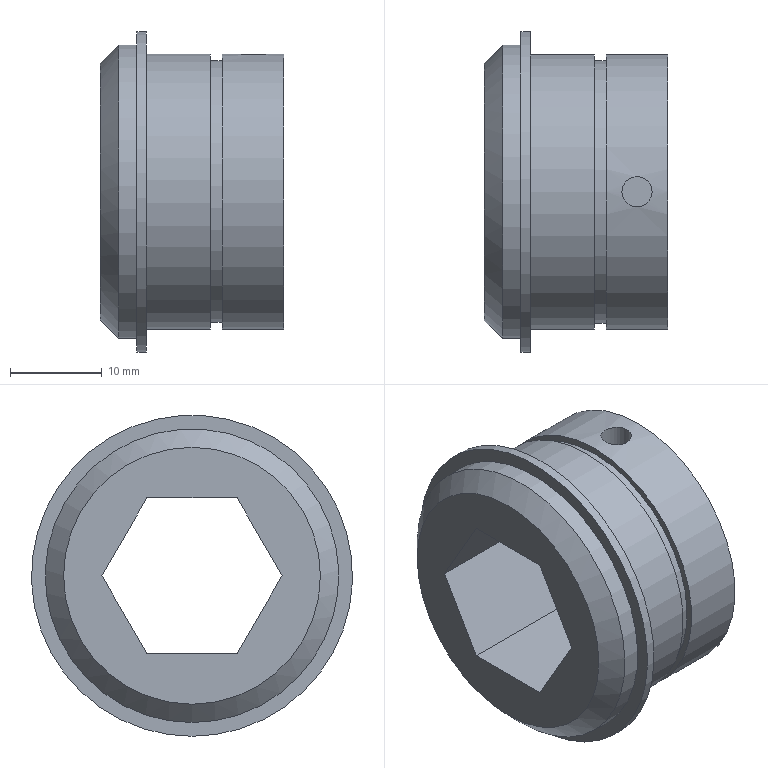Part | STEP file | Slotted wheel end cap | 1 solid | 19 faces | box 20 x 35 x 35 mm | volume 9444 mm3 | plane 12 | cylinder 6 | cone 1 | commonest cylinder face diameters 30 x2 3.3 x1 28.6 x1 32 x1 35 x1
STEP:
#1=CARTESIAN_POINT('',(5.,0.,-15.));
#2=VERTEX_POINT('',#1);
#3=CARTESIAN_POINT('',(5.,0.,0.));
#4=DIRECTION('',(1.,0.,0.));
#5=DIRECTION('',(0.,0.,-1.));
#6=AXIS2_PLACEMENT_3D('',#3,#4,#5);
#7=CIRCLE('',#6,15.);
#8=EDGE_CURVE('',#2,#2,#7,.T.);
#9=ORIENTED_EDGE('',*,*,#8,.T.);
#10=EDGE_LOOP('',(#9));
#11=FACE_OUTER_BOUND('',#10,.T.);
#12=CARTESIAN_POINT('',(12.,0.,15.));
#13=VERTEX_POINT('',#12);
#14=CARTESIAN_POINT('',(12.,0.,0.));
#15=DIRECTION('',(-1.,0.,0.));
#16=DIRECTION('',(0.,0.,1.));
#17=AXIS2_PLACEMENT_3D('',#14,#15,#16);
#18=CIRCLE('',#17,15.);
#19=EDGE_CURVE('',#13,#13,#18,.T.);
#20=ORIENTED_EDGE('',*,*,#19,.T.);
#21=EDGE_LOOP('',(#20));
#22=FACE_OUTER_BOUND('',#21,.T.);
#23=CARTESIAN_POINT('',(5.,0.,0.));
#24=DIRECTION('',(1.,0.,0.));
#25=DIRECTION('',(0.,0.,-1.));
#26=AXIS2_PLACEMENT_3D('',#23,#24,#25);
#27=CYLINDRICAL_SURFACE('',#26,15.);
#28=ADVANCED_FACE('',(#11,#22),#27,.T.);
#29=CARTESIAN_POINT('',(20.,0.,-15.));
#30=VERTEX_POINT('',#29);
#31=CARTESIAN_POINT('',(20.,0.,0.));
#32=DIRECTION('',(1.,0.,0.));
#33=DIRECTION('',(0.,0.,-1.));
#34=AXIS2_PLACEMENT_3D('',#31,#32,#33);
#35=CIRCLE('',#34,15.);
#36=EDGE_CURVE('',#30,#30,#35,.T.);
#37=ORIENTED_EDGE('',*,*,#36,.F.);
#38=EDGE_LOOP('',(#37));
#39=FACE_OUTER_BOUND('',#38,.T.);
#40=CARTESIAN_POINT('',(15.,0.,15.));
#41=VERTEX_POINT('',#40);
#42=CARTESIAN_POINT('',(15.,0.,15.));
#43=CARTESIAN_POINT('',(15.,-0.1091,15.));
#44=CARTESIAN_POINT('',(15.011,-0.2164,14.999));
#45=CARTESIAN_POINT('',(15.053,-0.4273,14.994));
#46=CARTESIAN_POINT('',(15.084,-0.5322,14.991));
#47=CARTESIAN_POINT('',(15.167,-0.7319,14.982));
#48=CARTESIAN_POINT('',(15.218,-0.8267,14.977));
#49=CARTESIAN_POINT('',(15.338,-1.006,14.966));
#50=CARTESIAN_POINT('',(15.407,-1.091,14.96));
#51=CARTESIAN_POINT('',(15.636,-1.319,14.943));
#52=CARTESIAN_POINT('',(15.819,-1.442,14.931));
#53=CARTESIAN_POINT('',(16.216,-1.606,14.914));
#54=CARTESIAN_POINT('',(16.434,-1.65,14.909));
#55=CARTESIAN_POINT('',(16.757,-1.65,14.909));
#56=CARTESIAN_POINT('',(16.866,-1.639,14.91));
#57=CARTESIAN_POINT('',(17.078,-1.597,14.915));
#58=CARTESIAN_POINT('',(17.181,-1.566,14.918));
#59=CARTESIAN_POINT('',(17.381,-1.483,14.927));
#60=CARTESIAN_POINT('',(17.477,-1.432,14.932));
#61=CARTESIAN_POINT('',(17.656,-1.312,14.943));
#62=CARTESIAN_POINT('',(17.739,-1.244,14.949));
#63=CARTESIAN_POINT('',(17.893,-1.09,14.961));
#64=CARTESIAN_POINT('',(17.961,-1.007,14.966));
#65=CARTESIAN_POINT('',(18.081,-0.8284,14.977));
#66=CARTESIAN_POINT('',(18.133,-0.7319,14.982));
#67=CARTESIAN_POINT('',(18.216,-0.5322,14.991));
#68=CARTESIAN_POINT('',(18.247,-0.4293,14.994));
#69=CARTESIAN_POINT('',(18.289,-0.2177,14.999));
#70=CARTESIAN_POINT('',(18.3,-0.1083,15.));
#71=CARTESIAN_POINT('',(18.3,0.2148,15.));
#72=CARTESIAN_POINT('',(18.257,0.4321,14.995));
#73=CARTESIAN_POINT('',(18.093,0.8293,14.978));
#74=CARTESIAN_POINT('',(17.97,1.013,14.967));
#75=CARTESIAN_POINT('',(17.742,1.242,14.949));
#76=CARTESIAN_POINT('',(17.657,1.311,14.943));
#77=CARTESIAN_POINT('',(17.478,1.431,14.932));
#78=CARTESIAN_POINT('',(17.383,1.482,14.927));
#79=CARTESIAN_POINT('',(17.184,1.565,14.918));
#80=CARTESIAN_POINT('',(17.079,1.597,14.915));
#81=CARTESIAN_POINT('',(16.868,1.639,14.91));
#82=CARTESIAN_POINT('',(16.761,1.65,14.909));
#83=CARTESIAN_POINT('',(16.542,1.65,14.909));
#84=CARTESIAN_POINT('',(16.435,1.639,14.91));
#85=CARTESIAN_POINT('',(16.224,1.598,14.915));
#86=CARTESIAN_POINT('',(16.119,1.566,14.918));
#87=CARTESIAN_POINT('',(15.919,1.483,14.927));
#88=CARTESIAN_POINT('',(15.825,1.433,14.932));
#89=CARTESIAN_POINT('',(15.645,1.313,14.943));
#90=CARTESIAN_POINT('',(15.56,1.244,14.949));
#91=CARTESIAN_POINT('',(15.332,1.016,14.966));
#92=CARTESIAN_POINT('',(15.209,0.8318,14.978));
#93=CARTESIAN_POINT('',(15.044,0.435,14.995));
#94=CARTESIAN_POINT('',(15.,0.2182,15.));
#95=CARTESIAN_POINT('',(15.,0.,15.));
#96=B_SPLINE_CURVE_WITH_KNOTS('',3,(#42,#43,#44,#45,#46,#47,#48,#49,#50,#51,#52,#53,#54,#55,#56,#57,#58,#59,#60,#61,#62,#63,#64,#65,#66,#67,#68,#69,#70,#71,#72,#73,#74,#75,#76,#77,#78,#79,#80,#81,#82,#83,#84,#85,#86,#87,#88,#89,#90,#91,#92,#93,#94,#95),.UNSPECIFIED.,.T.,.F.,(4,2,2,2,2,2,2,2,2,2,2,2,2,2,2,2,2,2,2,2,2,2,2,2,2,2,4),(0.,0.0003226,0.0006452,0.0009679,0.00129,0.001936,0.002581,0.002904,0.003226,0.003549,0.003871,0.004194,0.004517,0.004839,0.005162,0.005807,0.006452,0.006775,0.007098,0.00742,0.007743,0.008066,0.008388,0.008711,0.009033,0.009679,0.01032),.UNSPECIFIED.);
#97=EDGE_CURVE('',#41,#41,#96,.T.);
#98=ORIENTED_EDGE('',*,*,#97,.F.);
#99=EDGE_LOOP('',(#98));
#100=FACE_BOUND('',#99,.T.);
#101=CARTESIAN_POINT('',(13.3,0.,15.));
#102=VERTEX_POINT('',#101);
#103=CARTESIAN_POINT('',(13.3,0.,0.));
#104=DIRECTION('',(-1.,0.,0.));
#105=DIRECTION('',(0.,0.,1.));
#106=AXIS2_PLACEMENT_3D('',#103,#104,#105);
#107=CIRCLE('',#106,15.);
#108=EDGE_CURVE('',#102,#102,#107,.T.);
#109=ORIENTED_EDGE('',*,*,#108,.F.);
#110=EDGE_LOOP('',(#109));
#111=FACE_OUTER_BOUND('',#110,.T.);
#112=CARTESIAN_POINT('',(5.,0.,0.));
#113=DIRECTION('',(1.,0.,0.));
#114=DIRECTION('',(0.,0.,-1.));
#115=AXIS2_PLACEMENT_3D('',#112,#113,#114);
#116=CYLINDRICAL_SURFACE('',#115,15.);
#117=ADVANCED_FACE('',(#39,#100,#111),#116,.T.);
#118=CARTESIAN_POINT('',(4.,0.,-17.5));
#119=VERTEX_POINT('',#118);
#120=CARTESIAN_POINT('',(4.,0.,0.));
#121=DIRECTION('',(1.,0.,0.));
#122=DIRECTION('',(0.,0.,-1.));
#123=AXIS2_PLACEMENT_3D('',#120,#121,#122);
#124=CIRCLE('',#123,17.5);
#125=EDGE_CURVE('',#119,#119,#124,.T.);
#126=ORIENTED_EDGE('',*,*,#125,.T.);
#127=EDGE_LOOP('',(#126));
#128=FACE_OUTER_BOUND('',#127,.T.);
#129=CARTESIAN_POINT('',(5.,0.,-17.5));
#130=VERTEX_POINT('',#129);
#131=CARTESIAN_POINT('',(5.,0.,0.));
#132=DIRECTION('',(1.,0.,0.));
#133=DIRECTION('',(0.,0.,-1.));
#134=AXIS2_PLACEMENT_3D('',#131,#132,#133);
#135=CIRCLE('',#134,17.5);
#136=EDGE_CURVE('',#130,#130,#135,.T.);
#137=ORIENTED_EDGE('',*,*,#136,.F.);
#138=EDGE_LOOP('',(#137));
#139=FACE_OUTER_BOUND('',#138,.T.);
#140=CARTESIAN_POINT('',(20.,0.,0.));
#141=DIRECTION('',(-1.,0.,0.));
#142=DIRECTION('',(0.,0.,1.));
#143=AXIS2_PLACEMENT_3D('',#140,#141,#142);
#144=CYLINDRICAL_SURFACE('',#143,17.5);
#145=ADVANCED_FACE('',(#128,#139),#144,.T.);
#146=CARTESIAN_POINT('',(20.,-9.815,0.));
#147=VERTEX_POINT('',#146);
#148=CARTESIAN_POINT('',(20.,-4.907,-8.5));
#149=VERTEX_POINT('',#148);
#150=CARTESIAN_POINT('',(20.,-9.815,0.));
#151=DIRECTION('',(0.,0.5,-0.866));
#152=VECTOR('',#151,1000.);
#153=LINE('',#150,#152);
#154=EDGE_CURVE('',#147,#149,#153,.T.);
#155=ORIENTED_EDGE('',*,*,#154,.F.);
#156=CARTESIAN_POINT('',(20.,-4.907,8.5));
#157=VERTEX_POINT('',#156);
#158=CARTESIAN_POINT('',(20.,-4.907,8.5));
#159=DIRECTION('',(0.,-0.5,-0.866));
#160=VECTOR('',#159,1000.);
#161=LINE('',#158,#160);
#162=EDGE_CURVE('',#157,#147,#161,.T.);
#163=ORIENTED_EDGE('',*,*,#162,.F.);
#164=CARTESIAN_POINT('',(20.,4.907,8.5));
#165=VERTEX_POINT('',#164);
#166=CARTESIAN_POINT('',(20.,4.907,8.5));
#167=DIRECTION('',(0.,-1.,0.));
#168=VECTOR('',#167,1000.);
#169=LINE('',#166,#168);
#170=EDGE_CURVE('',#165,#157,#169,.T.);
#171=ORIENTED_EDGE('',*,*,#170,.F.);
#172=CARTESIAN_POINT('',(20.,9.815,0.));
#173=VERTEX_POINT('',#172);
#174=CARTESIAN_POINT('',(20.,9.815,0.));
#175=DIRECTION('',(0.,-0.5,0.866));
#176=VECTOR('',#175,1000.);
#177=LINE('',#174,#176);
#178=EDGE_CURVE('',#173,#165,#177,.T.);
#179=ORIENTED_EDGE('',*,*,#178,.F.);
#180=CARTESIAN_POINT('',(20.,4.907,-8.5));
#181=VERTEX_POINT('',#180);
#182=CARTESIAN_POINT('',(20.,4.907,-8.5));
#183=DIRECTION('',(0.,0.5,0.866));
#184=VECTOR('',#183,1000.);
#185=LINE('',#182,#184);
#186=EDGE_CURVE('',#181,#173,#185,.T.);
#187=ORIENTED_EDGE('',*,*,#186,.F.);
#188=CARTESIAN_POINT('',(20.,-4.907,-8.5));
#189=DIRECTION('',(0.,1.,0.));
#190=VECTOR('',#189,1000.);
#191=LINE('',#188,#190);
#192=EDGE_CURVE('',#149,#181,#191,.T.);
#193=ORIENTED_EDGE('',*,*,#192,.F.);
#194=EDGE_LOOP('',(#155,#163,#171,#179,#187,#193));
#195=FACE_BOUND('',#194,.T.);
#196=ORIENTED_EDGE('',*,*,#36,.T.);
#197=EDGE_LOOP('',(#196));
#198=FACE_OUTER_BOUND('',#197,.T.);
#199=CARTESIAN_POINT('',(20.,0.,0.));
#200=DIRECTION('',(1.,0.,0.));
#201=DIRECTION('',(0.,0.,-1.));
#202=AXIS2_PLACEMENT_3D('',#199,#200,#201);
#203=PLANE('',#202);
#204=ADVANCED_FACE('',(#195,#198),#203,.T.);
#205=CARTESIAN_POINT('',(2.,0.,-16.));
#206=VERTEX_POINT('',#205);
#207=CARTESIAN_POINT('',(2.,0.,0.));
#208=DIRECTION('',(1.,0.,0.));
#209=DIRECTION('',(0.,0.,-1.));
#210=AXIS2_PLACEMENT_3D('',#207,#208,#209);
#211=CIRCLE('',#210,16.);
#212=EDGE_CURVE('',#206,#206,#211,.T.);
#213=ORIENTED_EDGE('',*,*,#212,.T.);
#214=EDGE_LOOP('',(#213));
#215=FACE_OUTER_BOUND('',#214,.T.);
#216=CARTESIAN_POINT('',(4.,0.,-16.));
#217=VERTEX_POINT('',#216);
#218=CARTESIAN_POINT('',(4.,0.,0.));
#219=DIRECTION('',(1.,0.,0.));
#220=DIRECTION('',(0.,0.,-1.));
#221=AXIS2_PLACEMENT_3D('',#218,#219,#220);
#222=CIRCLE('',#221,16.);
#223=EDGE_CURVE('',#217,#217,#222,.T.);
#224=ORIENTED_EDGE('',*,*,#223,.F.);
#225=EDGE_LOOP('',(#224));
#226=FACE_OUTER_BOUND('',#225,.T.);
#227=CARTESIAN_POINT('',(4.,0.,0.));
#228=DIRECTION('',(-1.,0.,0.));
#229=DIRECTION('',(0.,0.,1.));
#230=AXIS2_PLACEMENT_3D('',#227,#228,#229);
#231=CYLINDRICAL_SURFACE('',#230,16.);
#232=ADVANCED_FACE('',(#215,#226),#231,.T.);
#233=CARTESIAN_POINT('',(0.,0.,-14.));
#234=VERTEX_POINT('',#233);
#235=CARTESIAN_POINT('',(0.,0.,0.));
#236=DIRECTION('',(-1.,0.,0.));
#237=DIRECTION('',(0.,0.,-1.));
#238=AXIS2_PLACEMENT_3D('',#235,#236,#237);
#239=CIRCLE('',#238,14.);
#240=EDGE_CURVE('',#234,#234,#239,.T.);
#241=ORIENTED_EDGE('',*,*,#240,.T.);
#242=EDGE_LOOP('',(#241));
#243=FACE_OUTER_BOUND('',#242,.T.);
#244=CARTESIAN_POINT('',(0.,-4.907,8.5));
#245=VERTEX_POINT('',#244);
#246=CARTESIAN_POINT('',(0.,-9.815,0.));
#247=VERTEX_POINT('',#246);
#248=CARTESIAN_POINT('',(0.,-4.907,8.5));
#249=DIRECTION('',(0.,-0.5,-0.866));
#250=VECTOR('',#249,1000.);
#251=LINE('',#248,#250);
#252=EDGE_CURVE('',#245,#247,#251,.T.);
#253=ORIENTED_EDGE('',*,*,#252,.T.);
#254=CARTESIAN_POINT('',(0.,-4.907,-8.5));
#255=VERTEX_POINT('',#254);
#256=CARTESIAN_POINT('',(0.,-9.815,0.));
#257=DIRECTION('',(0.,0.5,-0.866));
#258=VECTOR('',#257,1000.);
#259=LINE('',#256,#258);
#260=EDGE_CURVE('',#247,#255,#259,.T.);
#261=ORIENTED_EDGE('',*,*,#260,.T.);
#262=CARTESIAN_POINT('',(0.,4.907,-8.5));
#263=VERTEX_POINT('',#262);
#264=CARTESIAN_POINT('',(0.,-4.907,-8.5));
#265=DIRECTION('',(0.,1.,0.));
#266=VECTOR('',#265,1000.);
#267=LINE('',#264,#266);
#268=EDGE_CURVE('',#255,#263,#267,.T.);
#269=ORIENTED_EDGE('',*,*,#268,.T.);
#270=CARTESIAN_POINT('',(0.,9.815,0.));
#271=VERTEX_POINT('',#270);
#272=CARTESIAN_POINT('',(0.,4.907,-8.5));
#273=DIRECTION('',(0.,0.5,0.866));
#274=VECTOR('',#273,1000.);
#275=LINE('',#272,#274);
#276=EDGE_CURVE('',#263,#271,#275,.T.);
#277=ORIENTED_EDGE('',*,*,#276,.T.);
#278=CARTESIAN_POINT('',(0.,4.907,8.5));
#279=VERTEX_POINT('',#278);
#280=CARTESIAN_POINT('',(0.,9.815,0.));
#281=DIRECTION('',(0.,-0.5,0.866));
#282=VECTOR('',#281,1000.);
#283=LINE('',#280,#282);
#284=EDGE_CURVE('',#271,#279,#283,.T.);
#285=ORIENTED_EDGE('',*,*,#284,.T.);
#286=CARTESIAN_POINT('',(0.,4.907,8.5));
#287=DIRECTION('',(0.,-1.,0.));
#288=VECTOR('',#287,1000.);
#289=LINE('',#286,#288);
#290=EDGE_CURVE('',#279,#245,#289,.T.);
#291=ORIENTED_EDGE('',*,*,#290,.T.);
#292=EDGE_LOOP('',(#253,#261,#269,#277,#285,#291));
#293=FACE_BOUND('',#292,.T.);
#294=CARTESIAN_POINT('',(0.,0.,0.));
#295=DIRECTION('',(1.,0.,0.));
#296=DIRECTION('',(0.,0.,-1.));
#297=AXIS2_PLACEMENT_3D('',#294,#295,#296);
#298=PLANE('',#297);
#299=ADVANCED_FACE('',(#243,#293),#298,.F.);
#300=ORIENTED_EDGE('',*,*,#223,.T.);
#301=EDGE_LOOP('',(#300));
#302=FACE_BOUND('',#301,.T.);
#303=ORIENTED_EDGE('',*,*,#125,.F.);
#304=EDGE_LOOP('',(#303));
#305=FACE_OUTER_BOUND('',#304,.T.);
#306=CARTESIAN_POINT('',(4.,0.,0.));
#307=DIRECTION('',(1.,0.,0.));
#308=DIRECTION('',(0.,0.,-1.));
#309=AXIS2_PLACEMENT_3D('',#306,#307,#308);
#310=PLANE('',#309);
#311=ADVANCED_FACE('',(#302,#305),#310,.F.);
#312=ORIENTED_EDGE('',*,*,#154,.T.);
#313=CARTESIAN_POINT('',(0.,-4.907,-8.5));
#314=DIRECTION('',(1.,0.,0.));
#315=VECTOR('',#314,1000.);
#316=LINE('',#313,#315);
#317=EDGE_CURVE('',#255,#149,#316,.T.);
#318=ORIENTED_EDGE('',*,*,#317,.F.);
#319=ORIENTED_EDGE('',*,*,#260,.F.);
#320=CARTESIAN_POINT('',(0.,-9.815,0.));
#321=DIRECTION('',(1.,0.,0.));
#322=VECTOR('',#321,1000.);
#323=LINE('',#320,#322);
#324=EDGE_CURVE('',#247,#147,#323,.T.);
#325=ORIENTED_EDGE('',*,*,#324,.T.);
#326=EDGE_LOOP('',(#312,#318,#319,#325));
#327=FACE_OUTER_BOUND('',#326,.T.);
#328=CARTESIAN_POINT('',(0.,-9.815,0.));
#329=DIRECTION('',(0.,-0.866,-0.5));
#330=DIRECTION('',(0.,0.5,-0.866));
#331=AXIS2_PLACEMENT_3D('',#328,#329,#330);
#332=PLANE('',#331);
#333=ADVANCED_FACE('',(#327),#332,.F.);
#334=ORIENTED_EDGE('',*,*,#162,.T.);
#335=ORIENTED_EDGE('',*,*,#324,.F.);
#336=ORIENTED_EDGE('',*,*,#252,.F.);
#337=CARTESIAN_POINT('',(0.,-4.907,8.5));
#338=DIRECTION('',(1.,0.,0.));
#339=VECTOR('',#338,1000.);
#340=LINE('',#337,#339);
#341=EDGE_CURVE('',#245,#157,#340,.T.);
#342=ORIENTED_EDGE('',*,*,#341,.T.);
#343=EDGE_LOOP('',(#334,#335,#336,#342));
#344=FACE_OUTER_BOUND('',#343,.T.);
#345=CARTESIAN_POINT('',(0.,-4.907,8.5));
#346=DIRECTION('',(0.,-0.866,0.5));
#347=DIRECTION('',(0.,-0.5,-0.866));
#348=AXIS2_PLACEMENT_3D('',#345,#346,#347);
#349=PLANE('',#348);
#350=ADVANCED_FACE('',(#344),#349,.F.);
#351=CARTESIAN_POINT('',(15.,0.,8.5));
#352=VERTEX_POINT('',#351);
#353=CARTESIAN_POINT('',(16.65,0.,8.5));
#354=DIRECTION('',(0.,0.,-1.));
#355=DIRECTION('',(-1.,0.,0.));
#356=AXIS2_PLACEMENT_3D('',#353,#354,#355);
#357=CIRCLE('',#356,1.65);
#358=EDGE_CURVE('',#352,#352,#357,.T.);
#359=ORIENTED_EDGE('',*,*,#358,.F.);
#360=EDGE_LOOP('',(#359));
#361=FACE_BOUND('',#360,.T.);
#362=ORIENTED_EDGE('',*,*,#170,.T.);
#363=ORIENTED_EDGE('',*,*,#341,.F.);
#364=ORIENTED_EDGE('',*,*,#290,.F.);
#365=CARTESIAN_POINT('',(0.,4.907,8.5));
#366=DIRECTION('',(1.,0.,0.));
#367=VECTOR('',#366,1000.);
#368=LINE('',#365,#367);
#369=EDGE_CURVE('',#279,#165,#368,.T.);
#370=ORIENTED_EDGE('',*,*,#369,.T.);
#371=EDGE_LOOP('',(#362,#363,#364,#370));
#372=FACE_OUTER_BOUND('',#371,.T.);
#373=CARTESIAN_POINT('',(0.,4.907,8.5));
#374=DIRECTION('',(0.,0.,1.));
#375=DIRECTION('',(1.,0.,0.));
#376=AXIS2_PLACEMENT_3D('',#373,#374,#375);
#377=PLANE('',#376);
#378=ADVANCED_FACE('',(#361,#372),#377,.F.);
#379=ORIENTED_EDGE('',*,*,#178,.T.);
#380=ORIENTED_EDGE('',*,*,#369,.F.);
#381=ORIENTED_EDGE('',*,*,#284,.F.);
#382=CARTESIAN_POINT('',(0.,9.815,0.));
#383=DIRECTION('',(1.,0.,0.));
#384=VECTOR('',#383,1000.);
#385=LINE('',#382,#384);
#386=EDGE_CURVE('',#271,#173,#385,.T.);
#387=ORIENTED_EDGE('',*,*,#386,.T.);
#388=EDGE_LOOP('',(#379,#380,#381,#387));
#389=FACE_OUTER_BOUND('',#388,.T.);
#390=CARTESIAN_POINT('',(0.,9.815,0.));
#391=DIRECTION('',(0.,0.866,0.5));
#392=DIRECTION('',(0.,-0.5,0.866));
#393=AXIS2_PLACEMENT_3D('',#390,#391,#392);
#394=PLANE('',#393);
#395=ADVANCED_FACE('',(#389),#394,.F.);
#396=ORIENTED_EDGE('',*,*,#186,.T.);
#397=ORIENTED_EDGE('',*,*,#386,.F.);
#398=ORIENTED_EDGE('',*,*,#276,.F.);
#399=CARTESIAN_POINT('',(0.,4.907,-8.5));
#400=DIRECTION('',(1.,0.,0.));
#401=VECTOR('',#400,1000.);
#402=LINE('',#399,#401);
#403=EDGE_CURVE('',#263,#181,#402,.T.);
#404=ORIENTED_EDGE('',*,*,#403,.T.);
#405=EDGE_LOOP('',(#396,#397,#398,#404));
#406=FACE_OUTER_BOUND('',#405,.T.);
#407=CARTESIAN_POINT('',(0.,4.907,-8.5));
#408=DIRECTION('',(0.,0.866,-0.5));
#409=DIRECTION('',(0.,0.5,0.866));
#410=AXIS2_PLACEMENT_3D('',#407,#408,#409);
#411=PLANE('',#410);
#412=ADVANCED_FACE('',(#406),#411,.F.);
#413=ORIENTED_EDGE('',*,*,#192,.T.);
#414=ORIENTED_EDGE('',*,*,#403,.F.);
#415=ORIENTED_EDGE('',*,*,#268,.F.);
#416=ORIENTED_EDGE('',*,*,#317,.T.);
#417=EDGE_LOOP('',(#413,#414,#415,#416));
#418=FACE_OUTER_BOUND('',#417,.T.);
#419=CARTESIAN_POINT('',(0.,-4.907,-8.5));
#420=DIRECTION('',(0.,0.,-1.));
#421=DIRECTION('',(0.,1.,0.));
#422=AXIS2_PLACEMENT_3D('',#419,#420,#421);
#423=PLANE('',#422);
#424=ADVANCED_FACE('',(#418),#423,.F.);
#425=ORIENTED_EDGE('',*,*,#8,.F.);
#426=EDGE_LOOP('',(#425));
#427=FACE_BOUND('',#426,.T.);
#428=ORIENTED_EDGE('',*,*,#136,.T.);
#429=EDGE_LOOP('',(#428));
#430=FACE_OUTER_BOUND('',#429,.T.);
#431=CARTESIAN_POINT('',(5.,0.,0.));
#432=DIRECTION('',(1.,0.,0.));
#433=DIRECTION('',(0.,0.,-1.));
#434=AXIS2_PLACEMENT_3D('',#431,#432,#433);
#435=PLANE('',#434);
#436=ADVANCED_FACE('',(#427,#430),#435,.T.);
#437=ORIENTED_EDGE('',*,*,#97,.T.);
#438=EDGE_LOOP('',(#437));
#439=FACE_OUTER_BOUND('',#438,.T.);
#440=ORIENTED_EDGE('',*,*,#358,.T.);
#441=EDGE_LOOP('',(#440));
#442=FACE_OUTER_BOUND('',#441,.T.);
#443=CARTESIAN_POINT('',(16.65,0.,8.5));
#444=DIRECTION('',(0.,0.,-1.));
#445=DIRECTION('',(-1.,0.,0.));
#446=AXIS2_PLACEMENT_3D('',#443,#444,#445);
#447=CYLINDRICAL_SURFACE('',#446,1.65);
#448=ADVANCED_FACE('',(#439,#442),#447,.F.);
#449=CARTESIAN_POINT('',(12.,0.,14.3));
#450=VERTEX_POINT('',#449);
#451=CARTESIAN_POINT('',(12.,0.,0.));
#452=DIRECTION('',(-1.,0.,0.));
#453=DIRECTION('',(0.,0.,1.));
#454=AXIS2_PLACEMENT_3D('',#451,#452,#453);
#455=CIRCLE('',#454,14.3);
#456=EDGE_CURVE('',#450,#450,#455,.T.);
#457=ORIENTED_EDGE('',*,*,#456,.T.);
#458=EDGE_LOOP('',(#457));
#459=FACE_BOUND('',#458,.T.);
#460=ORIENTED_EDGE('',*,*,#19,.F.);
#461=EDGE_LOOP('',(#460));
#462=FACE_OUTER_BOUND('',#461,.T.);
#463=CARTESIAN_POINT('',(12.,15.,0.));
#464=DIRECTION('',(1.,0.,0.));
#465=DIRECTION('',(0.,0.,-1.));
#466=AXIS2_PLACEMENT_3D('',#463,#464,#465);
#467=PLANE('',#466);
#468=ADVANCED_FACE('',(#459,#462),#467,.T.);
#469=CARTESIAN_POINT('',(13.3,0.,14.3));
#470=VERTEX_POINT('',#469);
#471=CARTESIAN_POINT('',(13.3,0.,0.));
#472=DIRECTION('',(-1.,0.,0.));
#473=DIRECTION('',(0.,0.,1.));
#474=AXIS2_PLACEMENT_3D('',#471,#472,#473);
#475=CIRCLE('',#474,14.3);
#476=EDGE_CURVE('',#470,#470,#475,.T.);
#477=ORIENTED_EDGE('',*,*,#476,.T.);
#478=EDGE_LOOP('',(#477));
#479=FACE_OUTER_BOUND('',#478,.T.);
#480=ORIENTED_EDGE('',*,*,#456,.F.);
#481=EDGE_LOOP('',(#480));
#482=FACE_OUTER_BOUND('',#481,.T.);
#483=CARTESIAN_POINT('',(0.,0.,0.));
#484=DIRECTION('',(-1.,0.,0.));
#485=DIRECTION('',(0.,0.,1.));
#486=AXIS2_PLACEMENT_3D('',#483,#484,#485);
#487=CYLINDRICAL_SURFACE('',#486,14.3);
#488=ADVANCED_FACE('',(#479,#482),#487,.T.);
#489=ORIENTED_EDGE('',*,*,#108,.T.);
#490=EDGE_LOOP('',(#489));
#491=FACE_OUTER_BOUND('',#490,.T.);
#492=ORIENTED_EDGE('',*,*,#476,.F.);
#493=EDGE_LOOP('',(#492));
#494=FACE_BOUND('',#493,.T.);
#495=CARTESIAN_POINT('',(13.3,15.,0.));
#496=DIRECTION('',(-1.,0.,0.));
#497=DIRECTION('',(0.,0.,1.));
#498=AXIS2_PLACEMENT_3D('',#495,#496,#497);
#499=PLANE('',#498);
#500=ADVANCED_FACE('',(#491,#494),#499,.T.);
#501=ORIENTED_EDGE('',*,*,#240,.F.);
#502=EDGE_LOOP('',(#501));
#503=FACE_BOUND('',#502,.T.);
#504=ORIENTED_EDGE('',*,*,#212,.F.);
#505=EDGE_LOOP('',(#504));
#506=FACE_OUTER_BOUND('',#505,.T.);
#507=CARTESIAN_POINT('',(2.,0.,0.));
#508=DIRECTION('',(1.,0.,0.));
#509=DIRECTION('',(0.,0.,-1.));
#510=AXIS2_PLACEMENT_3D('',#507,#508,#509);
#511=CONICAL_SURFACE('',#510,16.,0.7854);
#512=ADVANCED_FACE('',(#503,#506),#511,.T.);
#513=CLOSED_SHELL('',(#28,#117,#145,#204,#232,#299,#311,#333,#350,#378,#395,#412,#424,#436,#448,#468,#488,#500,#512));
#514=MANIFOLD_SOLID_BREP('',#513);
#515=CARTESIAN_POINT('',(0.,0.,0.));
#516=DIRECTION('',(0.,0.,1.));
#517=DIRECTION('',(1.,0.,0.));
#518=AXIS2_PLACEMENT_3D('',#515,#516,#517);
#519=(LENGTH_UNIT()NAMED_UNIT(*)SI_UNIT(.MILLI.,.METRE.));
#520=UNCERTAINTY_MEASURE_WITH_UNIT(LENGTH_MEASURE(0.00001),#519,'','');
#521=(NAMED_UNIT(*)PLANE_ANGLE_UNIT()SI_UNIT($,.RADIAN.));
#522=(NAMED_UNIT(*)SI_UNIT($,.STERADIAN.)SOLID_ANGLE_UNIT());
#523=(GEOMETRIC_REPRESENTATION_CONTEXT(3)GLOBAL_UNCERTAINTY_ASSIGNED_CONTEXT((#520))GLOBAL_UNIT_ASSIGNED_CONTEXT((#519,#521,#522))REPRESENTATION_CONTEXT('',''));
#524=ADVANCED_BREP_SHAPE_REPRESENTATION('',(#514,#518),#523);